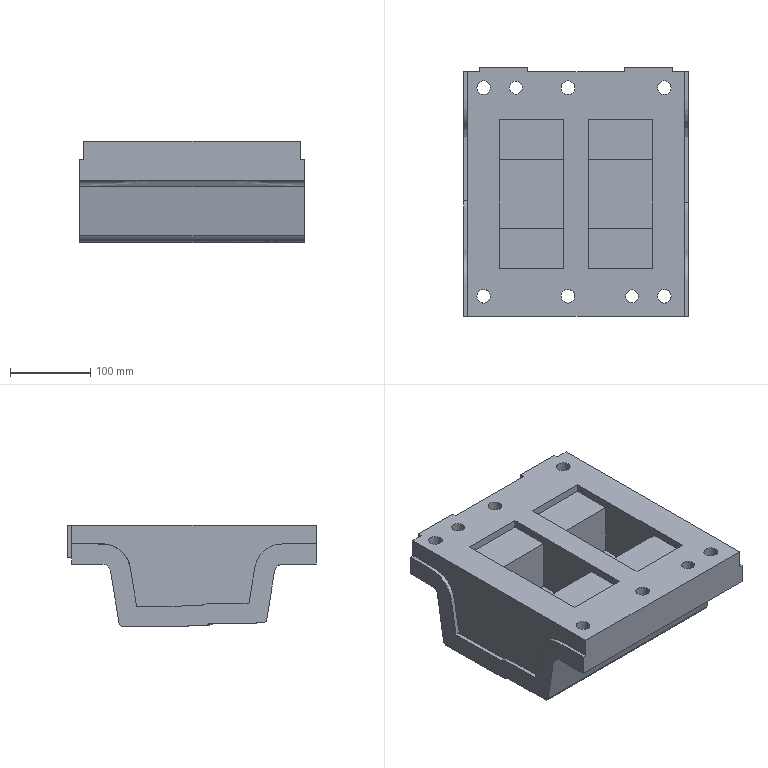Part | NX | features solid 2 | 1 solid | 85 faces | box 280.327 x 310 x 126.004 mm | volume 6807887 mm3 | plane 45 | spline 22 | cylinder 18 | commonest cylinder face diameters 17 x6 26 x6 10 x2 12 x2 16 x2